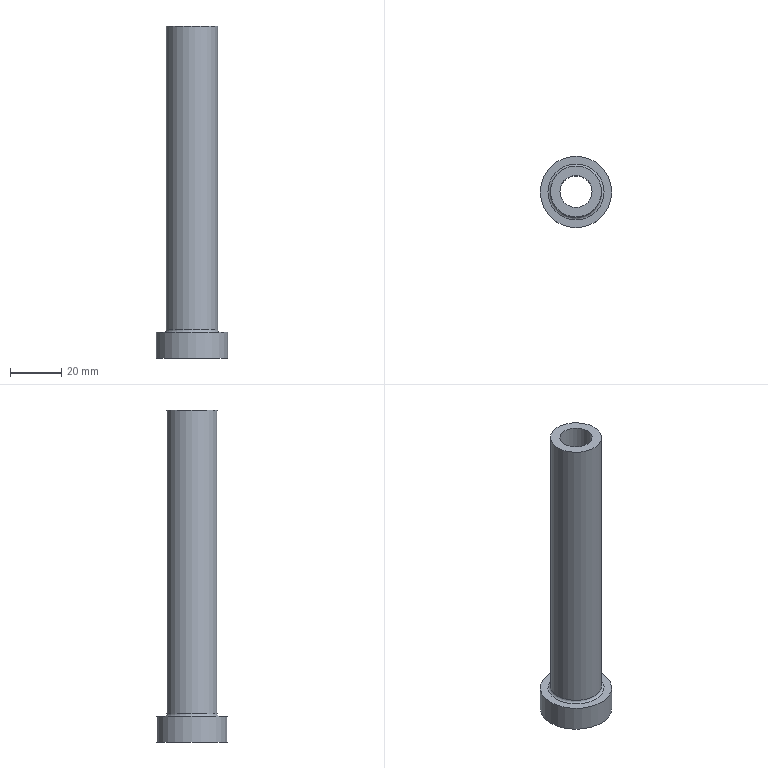Part | NX | features 19 2 | 1 solid | 7 faces | box 28 x 28 x 130 mm | volume 27661 mm3 | cylinder 3 | plane 3 | torus 1 | commonest cylinder face diameters 12.6 x1 20 x1 28 x1
STEP:
#1=CARTESIAN_POINT('',(867.,-315.,-38.5));
#2=VERTEX_POINT('',#1);
#3=CARTESIAN_POINT('',(877.,-315.,-38.5));
#4=DIRECTION('',(0.,0.,-1.));
#5=DIRECTION('',(-1.,0.,0.));
#6=AXIS2_PLACEMENT_3D('',#3,#4,#5);
#7=CIRCLE('',#6,10.);
#8=EDGE_CURVE('',#2,#2,#7,.T.);
#9=ORIENTED_EDGE('',*,*,#8,.T.);
#10=EDGE_LOOP('',(#9));
#11=FACE_BOUND('',#10,.T.);
#12=CARTESIAN_POINT('',(867.,-315.,-157.5));
#13=VERTEX_POINT('',#12);
#14=CARTESIAN_POINT('',(877.,-315.,-157.5));
#15=DIRECTION('',(0.,0.,1.));
#16=DIRECTION('',(1.,0.,0.));
#17=AXIS2_PLACEMENT_3D('',#14,#15,#16);
#18=CIRCLE('',#17,10.);
#19=EDGE_CURVE('',#13,#13,#18,.T.);
#20=ORIENTED_EDGE('',*,*,#19,.T.);
#21=EDGE_LOOP('',(#20));
#22=FACE_BOUND('',#21,.T.);
#23=CARTESIAN_POINT('',(877.,-315.,-88.5));
#24=DIRECTION('',(0.,0.,1.));
#25=DIRECTION('',(-1.,0.,0.));
#26=AXIS2_PLACEMENT_3D('',#23,#24,#25);
#27=CYLINDRICAL_SURFACE('',#26,10.);
#28=ADVANCED_FACE('',(#11,#22),#27,.T.);
#29=CARTESIAN_POINT('',(870.7,-315.,-168.5));
#30=VERTEX_POINT('',#29);
#31=CARTESIAN_POINT('',(877.,-315.,-168.5));
#32=DIRECTION('',(0.,0.,-1.));
#33=DIRECTION('',(-1.,0.,0.));
#34=AXIS2_PLACEMENT_3D('',#31,#32,#33);
#35=CIRCLE('',#34,6.3);
#36=EDGE_CURVE('',#30,#30,#35,.T.);
#37=ORIENTED_EDGE('',*,*,#36,.T.);
#38=EDGE_LOOP('',(#37));
#39=FACE_BOUND('',#38,.T.);
#40=CARTESIAN_POINT('',(870.7,-315.,-38.5));
#41=VERTEX_POINT('',#40);
#42=CARTESIAN_POINT('',(877.,-315.,-38.5));
#43=DIRECTION('',(0.,0.,1.));
#44=DIRECTION('',(-1.,0.,0.));
#45=AXIS2_PLACEMENT_3D('',#42,#43,#44);
#46=CIRCLE('',#45,6.3);
#47=EDGE_CURVE('',#41,#41,#46,.T.);
#48=ORIENTED_EDGE('',*,*,#47,.T.);
#49=EDGE_LOOP('',(#48));
#50=FACE_BOUND('',#49,.T.);
#51=CARTESIAN_POINT('',(877.,-315.,-93.5));
#52=DIRECTION('',(0.,0.,1.));
#53=DIRECTION('',(-1.,0.,0.));
#54=AXIS2_PLACEMENT_3D('',#51,#52,#53);
#55=CYLINDRICAL_SURFACE('',#54,6.3);
#56=ADVANCED_FACE('',(#39,#50),#55,.F.);
#57=ORIENTED_EDGE('',*,*,#19,.F.);
#58=EDGE_LOOP('',(#57));
#59=FACE_BOUND('',#58,.T.);
#60=CARTESIAN_POINT('',(866.,-315.,-158.5));
#61=VERTEX_POINT('',#60);
#62=CARTESIAN_POINT('',(877.,-315.,-158.5));
#63=DIRECTION('',(0.,0.,-1.));
#64=DIRECTION('',(1.,0.,0.));
#65=AXIS2_PLACEMENT_3D('',#62,#63,#64);
#66=CIRCLE('',#65,11.);
#67=EDGE_CURVE('',#61,#61,#66,.T.);
#68=ORIENTED_EDGE('',*,*,#67,.F.);
#69=EDGE_LOOP('',(#68));
#70=FACE_BOUND('',#69,.T.);
#71=CARTESIAN_POINT('',(877.,-315.,-157.5));
#72=DIRECTION('',(0.,0.,-1.));
#73=DIRECTION('',(1.,0.,0.));
#74=AXIS2_PLACEMENT_3D('',#71,#72,#73);
#75=TOROIDAL_SURFACE('',#74,11.,1.);
#76=ADVANCED_FACE('',(#59,#70),#75,.F.);
#77=CARTESIAN_POINT('',(863.,-315.,-158.5));
#78=VERTEX_POINT('',#77);
#79=CARTESIAN_POINT('',(877.,-315.,-158.5));
#80=DIRECTION('',(0.,0.,-1.));
#81=DIRECTION('',(-1.,0.,0.));
#82=AXIS2_PLACEMENT_3D('',#79,#80,#81);
#83=CIRCLE('',#82,14.);
#84=EDGE_CURVE('',#78,#78,#83,.T.);
#85=ORIENTED_EDGE('',*,*,#84,.F.);
#86=EDGE_LOOP('',(#85));
#87=FACE_BOUND('',#86,.T.);
#88=ORIENTED_EDGE('',*,*,#67,.T.);
#89=EDGE_LOOP('',(#88));
#90=FACE_BOUND('',#89,.T.);
#91=CARTESIAN_POINT('',(877.,-315.,-158.5));
#92=DIRECTION('',(0.,0.,1.));
#93=DIRECTION('',(-1.,0.,0.));
#94=AXIS2_PLACEMENT_3D('',#91,#92,#93);
#95=PLANE('',#94);
#96=ADVANCED_FACE('',(#87,#90),#95,.T.);
#97=ORIENTED_EDGE('',*,*,#47,.F.);
#98=EDGE_LOOP('',(#97));
#99=FACE_BOUND('',#98,.T.);
#100=ORIENTED_EDGE('',*,*,#8,.F.);
#101=EDGE_LOOP('',(#100));
#102=FACE_BOUND('',#101,.T.);
#103=CARTESIAN_POINT('',(877.,-315.,-38.5));
#104=DIRECTION('',(0.,0.,1.));
#105=DIRECTION('',(-1.,0.,0.));
#106=AXIS2_PLACEMENT_3D('',#103,#104,#105);
#107=PLANE('',#106);
#108=ADVANCED_FACE('',(#99,#102),#107,.T.);
#109=CARTESIAN_POINT('',(863.,-315.,-168.5));
#110=VERTEX_POINT('',#109);
#111=CARTESIAN_POINT('',(877.,-315.,-168.5));
#112=DIRECTION('',(0.,0.,1.));
#113=DIRECTION('',(-1.,0.,0.));
#114=AXIS2_PLACEMENT_3D('',#111,#112,#113);
#115=CIRCLE('',#114,14.);
#116=EDGE_CURVE('',#110,#110,#115,.T.);
#117=ORIENTED_EDGE('',*,*,#116,.T.);
#118=EDGE_LOOP('',(#117));
#119=FACE_BOUND('',#118,.T.);
#120=ORIENTED_EDGE('',*,*,#84,.T.);
#121=EDGE_LOOP('',(#120));
#122=FACE_BOUND('',#121,.T.);
#123=CARTESIAN_POINT('',(877.,-315.,-163.5));
#124=DIRECTION('',(0.,0.,1.));
#125=DIRECTION('',(-1.,0.,0.));
#126=AXIS2_PLACEMENT_3D('',#123,#124,#125);
#127=CYLINDRICAL_SURFACE('',#126,14.);
#128=ADVANCED_FACE('',(#119,#122),#127,.T.);
#129=ORIENTED_EDGE('',*,*,#36,.F.);
#130=EDGE_LOOP('',(#129));
#131=FACE_BOUND('',#130,.T.);
#132=ORIENTED_EDGE('',*,*,#116,.F.);
#133=EDGE_LOOP('',(#132));
#134=FACE_BOUND('',#133,.T.);
#135=CARTESIAN_POINT('',(877.,-315.,-168.5));
#136=DIRECTION('',(0.,0.,-1.));
#137=DIRECTION('',(1.,0.,0.));
#138=AXIS2_PLACEMENT_3D('',#135,#136,#137);
#139=PLANE('',#138);
#140=ADVANCED_FACE('',(#131,#134),#139,.T.);
#141=CLOSED_SHELL('',(#28,#56,#76,#96,#108,#128,#140));
#142=MANIFOLD_SOLID_BREP('',#141);
#143=(LENGTH_UNIT()NAMED_UNIT(*)SI_UNIT(.MILLI.,.METRE.));
#144=UNCERTAINTY_MEASURE_WITH_UNIT(LENGTH_MEASURE(0.00001),#143,'','');
#145=(NAMED_UNIT(*)PLANE_ANGLE_UNIT()SI_UNIT($,.RADIAN.));
#146=(NAMED_UNIT(*)SI_UNIT($,.STERADIAN.)SOLID_ANGLE_UNIT());
#147=(GEOMETRIC_REPRESENTATION_CONTEXT(3)GLOBAL_UNCERTAINTY_ASSIGNED_CONTEXT((#144))GLOBAL_UNIT_ASSIGNED_CONTEXT((#143,#145,#146))REPRESENTATION_CONTEXT('',''));
#148=ADVANCED_BREP_SHAPE_REPRESENTATION('',(#142),#147);